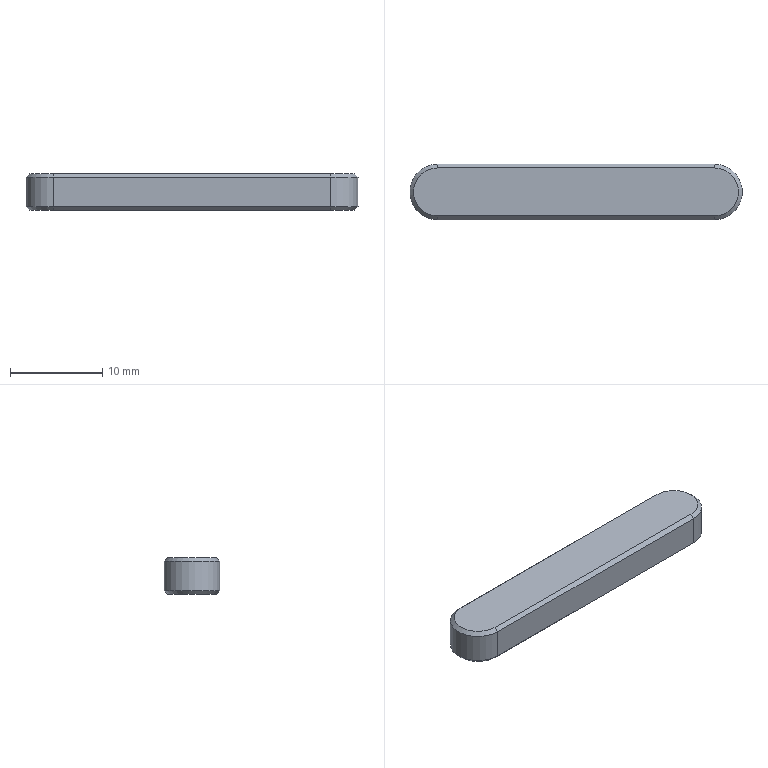Part | SolidWorks | features BaseBody 1 | 1 solid | 14 faces | box 36 x 6 x 4 mm | volume 820.615 mm3 | plane 8 | cone 4 | cylinder 2 | commonest cylinder face diameters 6 x2
STEP:
#1=CARTESIAN_POINT('',(33.,-2.6,-2.5));
#2=VERTEX_POINT('',#1);
#3=CARTESIAN_POINT('',(33.,-3.,-2.1));
#4=VERTEX_POINT('',#3);
#5=CARTESIAN_POINT('',(33.,-2.6,-2.5));
#6=DIRECTION('',(0.,-0.7071,0.7071));
#7=VECTOR('',#6,1000.);
#8=LINE('',#5,#7);
#9=EDGE_CURVE('',#2,#4,#8,.T.);
#10=ORIENTED_EDGE('',*,*,#9,.T.);
#11=CARTESIAN_POINT('',(3.,-3.,-2.1));
#12=VERTEX_POINT('',#11);
#13=CARTESIAN_POINT('',(10.5,-3.,-2.1));
#14=DIRECTION('',(-1.,0.,0.));
#15=VECTOR('',#14,1000.);
#16=LINE('',#13,#15);
#17=EDGE_CURVE('',#4,#12,#16,.T.);
#18=ORIENTED_EDGE('',*,*,#17,.T.);
#19=CARTESIAN_POINT('',(3.,-2.6,-2.5));
#20=VERTEX_POINT('',#19);
#21=CARTESIAN_POINT('',(3.,-3.,-2.1));
#22=DIRECTION('',(0.,0.7071,-0.7071));
#23=VECTOR('',#22,1000.);
#24=LINE('',#21,#23);
#25=EDGE_CURVE('',#12,#20,#24,.T.);
#26=ORIENTED_EDGE('',*,*,#25,.T.);
#27=CARTESIAN_POINT('',(10.5,-2.6,-2.5));
#28=DIRECTION('',(1.,0.,0.));
#29=VECTOR('',#28,1000.);
#30=LINE('',#27,#29);
#31=EDGE_CURVE('',#20,#2,#30,.T.);
#32=ORIENTED_EDGE('',*,*,#31,.T.);
#33=EDGE_LOOP('',(#10,#18,#26,#32));
#34=FACE_OUTER_BOUND('',#33,.T.);
#35=CARTESIAN_POINT('',(10.5,-2.8,-2.3));
#36=DIRECTION('',(0.,-0.7071,-0.7071));
#37=DIRECTION('',(0.,-0.7071,0.7071));
#38=AXIS2_PLACEMENT_3D('',#35,#36,#37);
#39=PLANE('',#38);
#40=ADVANCED_FACE('',(#34),#39,.T.);
#41=CARTESIAN_POINT('',(33.,2.6,-2.5));
#42=VERTEX_POINT('',#41);
#43=CARTESIAN_POINT('',(33.,3.,-2.1));
#44=VERTEX_POINT('',#43);
#45=CARTESIAN_POINT('',(33.,2.6,-2.5));
#46=DIRECTION('',(0.,0.7071,0.7071));
#47=VECTOR('',#46,1000.);
#48=LINE('',#45,#47);
#49=EDGE_CURVE('',#42,#44,#48,.T.);
#50=ORIENTED_EDGE('',*,*,#49,.T.);
#51=CARTESIAN_POINT('',(33.,0.,-2.1));
#52=DIRECTION('',(0.,0.,-1.));
#53=DIRECTION('',(0.,1.,0.));
#54=AXIS2_PLACEMENT_3D('',#51,#52,#53);
#55=CIRCLE('',#54,3.);
#56=EDGE_CURVE('',#44,#4,#55,.T.);
#57=ORIENTED_EDGE('',*,*,#56,.T.);
#58=ORIENTED_EDGE('',*,*,#9,.F.);
#59=CARTESIAN_POINT('',(33.,0.,-2.5));
#60=DIRECTION('',(0.,0.,1.));
#61=DIRECTION('',(0.,1.,0.));
#62=AXIS2_PLACEMENT_3D('',#59,#60,#61);
#63=CIRCLE('',#62,2.6);
#64=EDGE_CURVE('',#2,#42,#63,.T.);
#65=ORIENTED_EDGE('',*,*,#64,.T.);
#66=EDGE_LOOP('',(#50,#57,#58,#65));
#67=FACE_OUTER_BOUND('',#66,.T.);
#68=CARTESIAN_POINT('',(33.,0.,-2.3));
#69=DIRECTION('',(0.,0.,1.));
#70=DIRECTION('',(0.,1.,0.));
#71=AXIS2_PLACEMENT_3D('',#68,#69,#70);
#72=CONICAL_SURFACE('',#71,2.8,0.7854);
#73=ADVANCED_FACE('',(#67),#72,.T.);
#74=CARTESIAN_POINT('',(3.,3.,-2.1));
#75=VERTEX_POINT('',#74);
#76=CARTESIAN_POINT('',(3.,2.6,-2.5));
#77=VERTEX_POINT('',#76);
#78=CARTESIAN_POINT('',(3.,3.,-2.1));
#79=DIRECTION('',(0.,-0.7071,-0.7071));
#80=VECTOR('',#79,1000.);
#81=LINE('',#78,#80);
#82=EDGE_CURVE('',#75,#77,#81,.T.);
#83=ORIENTED_EDGE('',*,*,#82,.T.);
#84=CARTESIAN_POINT('',(3.,0.,-2.5));
#85=DIRECTION('',(0.,0.,1.));
#86=DIRECTION('',(0.,-1.,0.));
#87=AXIS2_PLACEMENT_3D('',#84,#85,#86);
#88=CIRCLE('',#87,2.6);
#89=EDGE_CURVE('',#77,#20,#88,.T.);
#90=ORIENTED_EDGE('',*,*,#89,.T.);
#91=ORIENTED_EDGE('',*,*,#25,.F.);
#92=CARTESIAN_POINT('',(3.,0.,-2.1));
#93=DIRECTION('',(0.,0.,-1.));
#94=DIRECTION('',(0.,-1.,0.));
#95=AXIS2_PLACEMENT_3D('',#92,#93,#94);
#96=CIRCLE('',#95,3.);
#97=EDGE_CURVE('',#12,#75,#96,.T.);
#98=ORIENTED_EDGE('',*,*,#97,.T.);
#99=EDGE_LOOP('',(#83,#90,#91,#98));
#100=FACE_OUTER_BOUND('',#99,.T.);
#101=CARTESIAN_POINT('',(3.,0.,-2.3));
#102=DIRECTION('',(0.,0.,1.));
#103=DIRECTION('',(0.,-1.,0.));
#104=AXIS2_PLACEMENT_3D('',#101,#102,#103);
#105=CONICAL_SURFACE('',#104,2.8,0.7854);
#106=ADVANCED_FACE('',(#100),#105,.T.);
#107=ORIENTED_EDGE('',*,*,#49,.F.);
#108=CARTESIAN_POINT('',(25.5,2.6,-2.5));
#109=DIRECTION('',(-1.,0.,0.));
#110=VECTOR('',#109,1000.);
#111=LINE('',#108,#110);
#112=EDGE_CURVE('',#42,#77,#111,.T.);
#113=ORIENTED_EDGE('',*,*,#112,.T.);
#114=ORIENTED_EDGE('',*,*,#82,.F.);
#115=CARTESIAN_POINT('',(25.5,3.,-2.1));
#116=DIRECTION('',(1.,0.,0.));
#117=VECTOR('',#116,1000.);
#118=LINE('',#115,#117);
#119=EDGE_CURVE('',#75,#44,#118,.T.);
#120=ORIENTED_EDGE('',*,*,#119,.T.);
#121=EDGE_LOOP('',(#107,#113,#114,#120));
#122=FACE_OUTER_BOUND('',#121,.T.);
#123=CARTESIAN_POINT('',(25.5,2.8,-2.3));
#124=DIRECTION('',(0.,0.7071,-0.7071));
#125=DIRECTION('',(-1.,0.,0.));
#126=AXIS2_PLACEMENT_3D('',#123,#124,#125);
#127=PLANE('',#126);
#128=ADVANCED_FACE('',(#122),#127,.T.);
#129=ORIENTED_EDGE('',*,*,#97,.F.);
#130=CARTESIAN_POINT('',(3.,-3.,1.1));
#131=VERTEX_POINT('',#130);
#132=CARTESIAN_POINT('',(3.,-3.,0.));
#133=DIRECTION('',(0.,0.,-1.));
#134=VECTOR('',#133,1000.);
#135=LINE('',#132,#134);
#136=EDGE_CURVE('',#131,#12,#135,.T.);
#137=ORIENTED_EDGE('',*,*,#136,.F.);
#138=CARTESIAN_POINT('',(3.,3.,1.1));
#139=VERTEX_POINT('',#138);
#140=CARTESIAN_POINT('',(3.,0.,1.1));
#141=DIRECTION('',(0.,0.,1.));
#142=DIRECTION('',(0.,-1.,0.));
#143=AXIS2_PLACEMENT_3D('',#140,#141,#142);
#144=CIRCLE('',#143,3.);
#145=EDGE_CURVE('',#139,#131,#144,.T.);
#146=ORIENTED_EDGE('',*,*,#145,.F.);
#147=CARTESIAN_POINT('',(3.,3.,0.));
#148=DIRECTION('',(0.,0.,1.));
#149=VECTOR('',#148,1000.);
#150=LINE('',#147,#149);
#151=EDGE_CURVE('',#75,#139,#150,.T.);
#152=ORIENTED_EDGE('',*,*,#151,.F.);
#153=EDGE_LOOP('',(#129,#137,#146,#152));
#154=FACE_OUTER_BOUND('',#153,.T.);
#155=CARTESIAN_POINT('',(3.,0.,0.));
#156=DIRECTION('',(0.,0.,1.));
#157=DIRECTION('',(0.,-1.,0.));
#158=AXIS2_PLACEMENT_3D('',#155,#156,#157);
#159=CYLINDRICAL_SURFACE('',#158,3.);
#160=ADVANCED_FACE('',(#154),#159,.T.);
#161=ORIENTED_EDGE('',*,*,#17,.F.);
#162=CARTESIAN_POINT('',(33.,-3.,1.1));
#163=VERTEX_POINT('',#162);
#164=CARTESIAN_POINT('',(33.,-3.,0.));
#165=DIRECTION('',(0.,0.,-1.));
#166=VECTOR('',#165,1000.);
#167=LINE('',#164,#166);
#168=EDGE_CURVE('',#163,#4,#167,.T.);
#169=ORIENTED_EDGE('',*,*,#168,.F.);
#170=CARTESIAN_POINT('',(10.5,-3.,1.1));
#171=DIRECTION('',(1.,0.,0.));
#172=VECTOR('',#171,1000.);
#173=LINE('',#170,#172);
#174=EDGE_CURVE('',#131,#163,#173,.T.);
#175=ORIENTED_EDGE('',*,*,#174,.F.);
#176=ORIENTED_EDGE('',*,*,#136,.T.);
#177=EDGE_LOOP('',(#161,#169,#175,#176));
#178=FACE_OUTER_BOUND('',#177,.T.);
#179=CARTESIAN_POINT('',(3.,-3.,0.));
#180=DIRECTION('',(0.,-1.,0.));
#181=DIRECTION('',(0.,0.,-1.));
#182=AXIS2_PLACEMENT_3D('',#179,#180,#181);
#183=PLANE('',#182);
#184=ADVANCED_FACE('',(#178),#183,.T.);
#185=ORIENTED_EDGE('',*,*,#31,.F.);
#186=ORIENTED_EDGE('',*,*,#89,.F.);
#187=ORIENTED_EDGE('',*,*,#112,.F.);
#188=ORIENTED_EDGE('',*,*,#64,.F.);
#189=EDGE_LOOP('',(#185,#186,#187,#188));
#190=FACE_OUTER_BOUND('',#189,.T.);
#191=CARTESIAN_POINT('',(18.,0.,-2.5));
#192=DIRECTION('',(0.,0.,1.));
#193=DIRECTION('',(1.,0.,0.));
#194=AXIS2_PLACEMENT_3D('',#191,#192,#193);
#195=PLANE('',#194);
#196=ADVANCED_FACE('',(#190),#195,.F.);
#197=CARTESIAN_POINT('',(3.,-2.6,1.5));
#198=VERTEX_POINT('',#197);
#199=CARTESIAN_POINT('',(3.,-3.,1.1));
#200=DIRECTION('',(0.,0.7071,0.7071));
#201=VECTOR('',#200,1000.);
#202=LINE('',#199,#201);
#203=EDGE_CURVE('',#131,#198,#202,.T.);
#204=ORIENTED_EDGE('',*,*,#203,.T.);
#205=CARTESIAN_POINT('',(3.,2.6,1.5));
#206=VERTEX_POINT('',#205);
#207=CARTESIAN_POINT('',(3.,0.,1.5));
#208=DIRECTION('',(0.,0.,-1.));
#209=DIRECTION('',(0.,-1.,0.));
#210=AXIS2_PLACEMENT_3D('',#207,#208,#209);
#211=CIRCLE('',#210,2.6);
#212=EDGE_CURVE('',#198,#206,#211,.T.);
#213=ORIENTED_EDGE('',*,*,#212,.T.);
#214=CARTESIAN_POINT('',(3.,2.6,1.5));
#215=DIRECTION('',(0.,0.7071,-0.7071));
#216=VECTOR('',#215,1000.);
#217=LINE('',#214,#216);
#218=EDGE_CURVE('',#206,#139,#217,.T.);
#219=ORIENTED_EDGE('',*,*,#218,.T.);
#220=ORIENTED_EDGE('',*,*,#145,.T.);
#221=EDGE_LOOP('',(#204,#213,#219,#220));
#222=FACE_OUTER_BOUND('',#221,.T.);
#223=CARTESIAN_POINT('',(3.,0.,1.3));
#224=DIRECTION('',(0.,0.,-1.));
#225=DIRECTION('',(0.,-1.,0.));
#226=AXIS2_PLACEMENT_3D('',#223,#224,#225);
#227=CONICAL_SURFACE('',#226,2.8,0.7854);
#228=ADVANCED_FACE('',(#222),#227,.T.);
#229=CARTESIAN_POINT('',(33.,-2.6,1.5));
#230=VERTEX_POINT('',#229);
#231=CARTESIAN_POINT('',(33.,-3.,1.1));
#232=DIRECTION('',(0.,0.7071,0.7071));
#233=VECTOR('',#232,1000.);
#234=LINE('',#231,#233);
#235=EDGE_CURVE('',#163,#230,#234,.T.);
#236=ORIENTED_EDGE('',*,*,#235,.T.);
#237=CARTESIAN_POINT('',(10.5,-2.6,1.5));
#238=DIRECTION('',(-1.,0.,0.));
#239=VECTOR('',#238,1000.);
#240=LINE('',#237,#239);
#241=EDGE_CURVE('',#230,#198,#240,.T.);
#242=ORIENTED_EDGE('',*,*,#241,.T.);
#243=ORIENTED_EDGE('',*,*,#203,.F.);
#244=ORIENTED_EDGE('',*,*,#174,.T.);
#245=EDGE_LOOP('',(#236,#242,#243,#244));
#246=FACE_OUTER_BOUND('',#245,.T.);
#247=CARTESIAN_POINT('',(10.5,-2.8,1.3));
#248=DIRECTION('',(0.,-0.7071,0.7071));
#249=DIRECTION('',(-1.,0.,0.));
#250=AXIS2_PLACEMENT_3D('',#247,#248,#249);
#251=PLANE('',#250);
#252=ADVANCED_FACE('',(#246),#251,.T.);
#253=CARTESIAN_POINT('',(33.,2.6,1.5));
#254=VERTEX_POINT('',#253);
#255=CARTESIAN_POINT('',(33.,3.,1.1));
#256=VERTEX_POINT('',#255);
#257=CARTESIAN_POINT('',(33.,2.6,1.5));
#258=DIRECTION('',(0.,0.7071,-0.7071));
#259=VECTOR('',#258,1000.);
#260=LINE('',#257,#259);
#261=EDGE_CURVE('',#254,#256,#260,.T.);
#262=ORIENTED_EDGE('',*,*,#261,.T.);
#263=CARTESIAN_POINT('',(25.5,3.,1.1));
#264=DIRECTION('',(-1.,0.,0.));
#265=VECTOR('',#264,1000.);
#266=LINE('',#263,#265);
#267=EDGE_CURVE('',#256,#139,#266,.T.);
#268=ORIENTED_EDGE('',*,*,#267,.T.);
#269=ORIENTED_EDGE('',*,*,#218,.F.);
#270=CARTESIAN_POINT('',(25.5,2.6,1.5));
#271=DIRECTION('',(1.,0.,0.));
#272=VECTOR('',#271,1000.);
#273=LINE('',#270,#272);
#274=EDGE_CURVE('',#206,#254,#273,.T.);
#275=ORIENTED_EDGE('',*,*,#274,.T.);
#276=EDGE_LOOP('',(#262,#268,#269,#275));
#277=FACE_OUTER_BOUND('',#276,.T.);
#278=CARTESIAN_POINT('',(25.5,2.8,1.3));
#279=DIRECTION('',(0.,0.7071,0.7071));
#280=DIRECTION('',(1.,0.,0.));
#281=AXIS2_PLACEMENT_3D('',#278,#279,#280);
#282=PLANE('',#281);
#283=ADVANCED_FACE('',(#277),#282,.T.);
#284=ORIENTED_EDGE('',*,*,#235,.F.);
#285=CARTESIAN_POINT('',(33.,0.,1.1));
#286=DIRECTION('',(0.,0.,1.));
#287=DIRECTION('',(0.,1.,0.));
#288=AXIS2_PLACEMENT_3D('',#285,#286,#287);
#289=CIRCLE('',#288,3.);
#290=EDGE_CURVE('',#163,#256,#289,.T.);
#291=ORIENTED_EDGE('',*,*,#290,.T.);
#292=ORIENTED_EDGE('',*,*,#261,.F.);
#293=CARTESIAN_POINT('',(33.,0.,1.5));
#294=DIRECTION('',(0.,0.,-1.));
#295=DIRECTION('',(0.,1.,0.));
#296=AXIS2_PLACEMENT_3D('',#293,#294,#295);
#297=CIRCLE('',#296,2.6);
#298=EDGE_CURVE('',#254,#230,#297,.T.);
#299=ORIENTED_EDGE('',*,*,#298,.T.);
#300=EDGE_LOOP('',(#284,#291,#292,#299));
#301=FACE_OUTER_BOUND('',#300,.T.);
#302=CARTESIAN_POINT('',(33.,0.,1.3));
#303=DIRECTION('',(0.,0.,-1.));
#304=DIRECTION('',(0.,1.,0.));
#305=AXIS2_PLACEMENT_3D('',#302,#303,#304);
#306=CONICAL_SURFACE('',#305,2.8,0.7854);
#307=ADVANCED_FACE('',(#301),#306,.T.);
#308=ORIENTED_EDGE('',*,*,#212,.F.);
#309=ORIENTED_EDGE('',*,*,#241,.F.);
#310=ORIENTED_EDGE('',*,*,#298,.F.);
#311=ORIENTED_EDGE('',*,*,#274,.F.);
#312=EDGE_LOOP('',(#308,#309,#310,#311));
#313=FACE_OUTER_BOUND('',#312,.T.);
#314=CARTESIAN_POINT('',(18.,0.,1.5));
#315=DIRECTION('',(0.,0.,1.));
#316=DIRECTION('',(1.,0.,0.));
#317=AXIS2_PLACEMENT_3D('',#314,#315,#316);
#318=PLANE('',#317);
#319=ADVANCED_FACE('',(#313),#318,.T.);
#320=ORIENTED_EDGE('',*,*,#119,.F.);
#321=ORIENTED_EDGE('',*,*,#151,.T.);
#322=ORIENTED_EDGE('',*,*,#267,.F.);
#323=CARTESIAN_POINT('',(33.,3.,0.));
#324=DIRECTION('',(0.,0.,-1.));
#325=VECTOR('',#324,1000.);
#326=LINE('',#323,#325);
#327=EDGE_CURVE('',#256,#44,#326,.T.);
#328=ORIENTED_EDGE('',*,*,#327,.T.);
#329=EDGE_LOOP('',(#320,#321,#322,#328));
#330=FACE_OUTER_BOUND('',#329,.T.);
#331=CARTESIAN_POINT('',(33.,3.,0.));
#332=DIRECTION('',(0.,1.,0.));
#333=DIRECTION('',(1.,0.,0.));
#334=AXIS2_PLACEMENT_3D('',#331,#332,#333);
#335=PLANE('',#334);
#336=ADVANCED_FACE('',(#330),#335,.T.);
#337=ORIENTED_EDGE('',*,*,#56,.F.);
#338=ORIENTED_EDGE('',*,*,#327,.F.);
#339=ORIENTED_EDGE('',*,*,#290,.F.);
#340=ORIENTED_EDGE('',*,*,#168,.T.);
#341=EDGE_LOOP('',(#337,#338,#339,#340));
#342=FACE_OUTER_BOUND('',#341,.T.);
#343=CARTESIAN_POINT('',(33.,0.,0.));
#344=DIRECTION('',(0.,0.,1.));
#345=DIRECTION('',(0.,1.,0.));
#346=AXIS2_PLACEMENT_3D('',#343,#344,#345);
#347=CYLINDRICAL_SURFACE('',#346,3.);
#348=ADVANCED_FACE('',(#342),#347,.T.);
#349=CLOSED_SHELL('',(#40,#73,#106,#128,#160,#184,#196,#228,#252,#283,#307,#319,#336,#348));
#350=MANIFOLD_SOLID_BREP('',#349);
#351=CARTESIAN_POINT('',(0.,0.,0.));
#352=DIRECTION('',(0.,0.,1.));
#353=DIRECTION('',(1.,0.,0.));
#354=AXIS2_PLACEMENT_3D('',#351,#352,#353);
#355=(LENGTH_UNIT()NAMED_UNIT(*)SI_UNIT(.MILLI.,.METRE.));
#356=UNCERTAINTY_MEASURE_WITH_UNIT(LENGTH_MEASURE(0.00001),#355,'','');
#357=(NAMED_UNIT(*)PLANE_ANGLE_UNIT()SI_UNIT($,.RADIAN.));
#358=(NAMED_UNIT(*)SI_UNIT($,.STERADIAN.)SOLID_ANGLE_UNIT());
#359=(GEOMETRIC_REPRESENTATION_CONTEXT(3)GLOBAL_UNCERTAINTY_ASSIGNED_CONTEXT((#356))GLOBAL_UNIT_ASSIGNED_CONTEXT((#355,#357,#358))REPRESENTATION_CONTEXT('',''));
#360=ADVANCED_BREP_SHAPE_REPRESENTATION('',(#350,#354),#359);